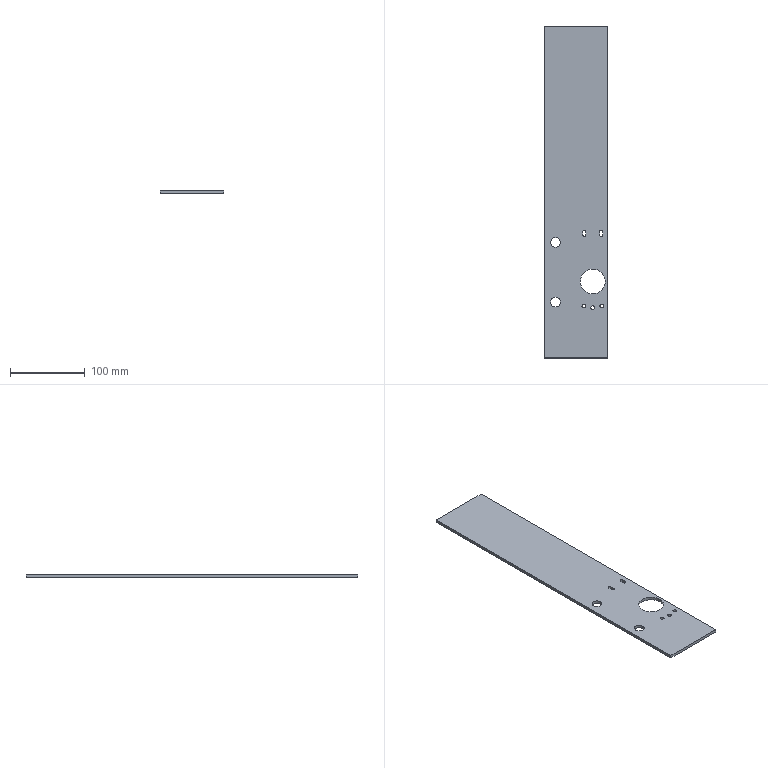Part | SolidWorks | features Extrusion 1 | 1 solid | 26 faces | box 85 x 445 x 4 mm | volume 146216 mm3 | cylinder 16 | plane 10 | commonest cylinder face diameters 5 x6 4 x4 13 x4 33.5 x2
STEP:
#1=CARTESIAN_POINT('',(48.25,-342.5,4.));
#2=VERTEX_POINT('',#1);
#3=CARTESIAN_POINT('',(81.75,-342.5,4.));
#4=VERTEX_POINT('',#3);
#5=CARTESIAN_POINT('',(65.,-342.5,4.));
#6=DIRECTION('',(0.,0.,1.));
#7=DIRECTION('',(1.,0.,0.));
#8=AXIS2_PLACEMENT_3D('',#5,#6,#7);
#9=CIRCLE('',#8,16.75);
#10=EDGE_CURVE('',#2,#4,#9,.T.);
#11=ORIENTED_EDGE('',*,*,#10,.T.);
#12=CARTESIAN_POINT('',(81.75,-342.5,0.));
#13=VERTEX_POINT('',#12);
#14=CARTESIAN_POINT('',(81.75,-342.5,4.));
#15=DIRECTION('',(0.,0.,-1.));
#16=VECTOR('',#15,1000.);
#17=LINE('',#14,#16);
#18=EDGE_CURVE('',#4,#13,#17,.T.);
#19=ORIENTED_EDGE('',*,*,#18,.T.);
#20=CARTESIAN_POINT('',(48.25,-342.5,0.));
#21=VERTEX_POINT('',#20);
#22=CARTESIAN_POINT('',(65.,-342.5,0.));
#23=DIRECTION('',(0.,0.,1.));
#24=DIRECTION('',(1.,0.,0.));
#25=AXIS2_PLACEMENT_3D('',#22,#23,#24);
#26=CIRCLE('',#25,16.75);
#27=EDGE_CURVE('',#21,#13,#26,.T.);
#28=ORIENTED_EDGE('',*,*,#27,.F.);
#29=CARTESIAN_POINT('',(48.25,-342.5,4.));
#30=DIRECTION('',(0.,0.,-1.));
#31=VECTOR('',#30,1000.);
#32=LINE('',#29,#31);
#33=EDGE_CURVE('',#2,#21,#32,.T.);
#34=ORIENTED_EDGE('',*,*,#33,.F.);
#35=EDGE_LOOP('',(#11,#19,#28,#34));
#36=FACE_OUTER_BOUND('',#35,.T.);
#37=CARTESIAN_POINT('',(65.,-342.5,4.));
#38=DIRECTION('',(0.,0.,-1.));
#39=DIRECTION('',(-1.,0.,0.));
#40=AXIS2_PLACEMENT_3D('',#37,#38,#39);
#41=CYLINDRICAL_SURFACE('',#40,16.75);
#42=ADVANCED_FACE('',(#36),#41,.F.);
#43=CARTESIAN_POINT('',(50.529,-375.389,4.));
#44=VERTEX_POINT('',#43);
#45=CARTESIAN_POINT('',(55.529,-375.389,4.));
#46=VERTEX_POINT('',#45);
#47=CARTESIAN_POINT('',(53.029,-375.389,4.));
#48=DIRECTION('',(0.,0.,1.));
#49=DIRECTION('',(1.,0.,0.));
#50=AXIS2_PLACEMENT_3D('',#47,#48,#49);
#51=CIRCLE('',#50,2.5);
#52=EDGE_CURVE('',#44,#46,#51,.T.);
#53=ORIENTED_EDGE('',*,*,#52,.T.);
#54=CARTESIAN_POINT('',(55.529,-375.389,0.));
#55=VERTEX_POINT('',#54);
#56=CARTESIAN_POINT('',(55.529,-375.389,4.));
#57=DIRECTION('',(0.,0.,-1.));
#58=VECTOR('',#57,1000.);
#59=LINE('',#56,#58);
#60=EDGE_CURVE('',#46,#55,#59,.T.);
#61=ORIENTED_EDGE('',*,*,#60,.T.);
#62=CARTESIAN_POINT('',(50.529,-375.389,0.));
#63=VERTEX_POINT('',#62);
#64=CARTESIAN_POINT('',(53.029,-375.389,0.));
#65=DIRECTION('',(0.,0.,1.));
#66=DIRECTION('',(1.,0.,0.));
#67=AXIS2_PLACEMENT_3D('',#64,#65,#66);
#68=CIRCLE('',#67,2.5);
#69=EDGE_CURVE('',#63,#55,#68,.T.);
#70=ORIENTED_EDGE('',*,*,#69,.F.);
#71=CARTESIAN_POINT('',(50.529,-375.389,4.));
#72=DIRECTION('',(0.,0.,-1.));
#73=VECTOR('',#72,1000.);
#74=LINE('',#71,#73);
#75=EDGE_CURVE('',#44,#63,#74,.T.);
#76=ORIENTED_EDGE('',*,*,#75,.F.);
#77=EDGE_LOOP('',(#53,#61,#70,#76));
#78=FACE_OUTER_BOUND('',#77,.T.);
#79=CARTESIAN_POINT('',(53.029,-375.389,4.));
#80=DIRECTION('',(0.,0.,-1.));
#81=DIRECTION('',(-1.,0.,0.));
#82=AXIS2_PLACEMENT_3D('',#79,#80,#81);
#83=CYLINDRICAL_SURFACE('',#82,2.5);
#84=ADVANCED_FACE('',(#78),#83,.F.);
#85=CARTESIAN_POINT('',(8.5,-290.,4.));
#86=VERTEX_POINT('',#85);
#87=CARTESIAN_POINT('',(21.5,-290.,4.));
#88=VERTEX_POINT('',#87);
#89=CARTESIAN_POINT('',(15.,-290.,4.));
#90=DIRECTION('',(0.,0.,1.));
#91=DIRECTION('',(1.,0.,0.));
#92=AXIS2_PLACEMENT_3D('',#89,#90,#91);
#93=CIRCLE('',#92,6.5);
#94=EDGE_CURVE('',#86,#88,#93,.T.);
#95=ORIENTED_EDGE('',*,*,#94,.T.);
#96=CARTESIAN_POINT('',(21.5,-290.,0.));
#97=VERTEX_POINT('',#96);
#98=CARTESIAN_POINT('',(21.5,-290.,4.));
#99=DIRECTION('',(0.,0.,-1.));
#100=VECTOR('',#99,1000.);
#101=LINE('',#98,#100);
#102=EDGE_CURVE('',#88,#97,#101,.T.);
#103=ORIENTED_EDGE('',*,*,#102,.T.);
#104=CARTESIAN_POINT('',(8.5,-290.,0.));
#105=VERTEX_POINT('',#104);
#106=CARTESIAN_POINT('',(15.,-290.,0.));
#107=DIRECTION('',(0.,0.,1.));
#108=DIRECTION('',(1.,0.,0.));
#109=AXIS2_PLACEMENT_3D('',#106,#107,#108);
#110=CIRCLE('',#109,6.5);
#111=EDGE_CURVE('',#105,#97,#110,.T.);
#112=ORIENTED_EDGE('',*,*,#111,.F.);
#113=CARTESIAN_POINT('',(8.5,-290.,4.));
#114=DIRECTION('',(0.,0.,-1.));
#115=VECTOR('',#114,1000.);
#116=LINE('',#113,#115);
#117=EDGE_CURVE('',#86,#105,#116,.T.);
#118=ORIENTED_EDGE('',*,*,#117,.F.);
#119=EDGE_LOOP('',(#95,#103,#112,#118));
#120=FACE_OUTER_BOUND('',#119,.T.);
#121=CARTESIAN_POINT('',(15.,-290.,4.));
#122=DIRECTION('',(0.,0.,-1.));
#123=DIRECTION('',(-1.,0.,0.));
#124=AXIS2_PLACEMENT_3D('',#121,#122,#123);
#125=CYLINDRICAL_SURFACE('',#124,6.5);
#126=ADVANCED_FACE('',(#120),#125,.F.);
#127=CARTESIAN_POINT('',(62.5,-377.5,4.));
#128=VERTEX_POINT('',#127);
#129=CARTESIAN_POINT('',(67.5,-377.5,4.));
#130=VERTEX_POINT('',#129);
#131=CARTESIAN_POINT('',(65.,-377.5,4.));
#132=DIRECTION('',(0.,0.,1.));
#133=DIRECTION('',(1.,0.,0.));
#134=AXIS2_PLACEMENT_3D('',#131,#132,#133);
#135=CIRCLE('',#134,2.5);
#136=EDGE_CURVE('',#128,#130,#135,.T.);
#137=ORIENTED_EDGE('',*,*,#136,.T.);
#138=CARTESIAN_POINT('',(67.5,-377.5,0.));
#139=VERTEX_POINT('',#138);
#140=CARTESIAN_POINT('',(67.5,-377.5,4.));
#141=DIRECTION('',(0.,0.,-1.));
#142=VECTOR('',#141,1000.);
#143=LINE('',#140,#142);
#144=EDGE_CURVE('',#130,#139,#143,.T.);
#145=ORIENTED_EDGE('',*,*,#144,.T.);
#146=CARTESIAN_POINT('',(62.5,-377.5,0.));
#147=VERTEX_POINT('',#146);
#148=CARTESIAN_POINT('',(65.,-377.5,0.));
#149=DIRECTION('',(0.,0.,1.));
#150=DIRECTION('',(1.,0.,0.));
#151=AXIS2_PLACEMENT_3D('',#148,#149,#150);
#152=CIRCLE('',#151,2.5);
#153=EDGE_CURVE('',#147,#139,#152,.T.);
#154=ORIENTED_EDGE('',*,*,#153,.F.);
#155=CARTESIAN_POINT('',(62.5,-377.5,4.));
#156=DIRECTION('',(0.,0.,-1.));
#157=VECTOR('',#156,1000.);
#158=LINE('',#155,#157);
#159=EDGE_CURVE('',#128,#147,#158,.T.);
#160=ORIENTED_EDGE('',*,*,#159,.F.);
#161=EDGE_LOOP('',(#137,#145,#154,#160));
#162=FACE_OUTER_BOUND('',#161,.T.);
#163=CARTESIAN_POINT('',(65.,-377.5,4.));
#164=DIRECTION('',(0.,0.,-1.));
#165=DIRECTION('',(-1.,0.,0.));
#166=AXIS2_PLACEMENT_3D('',#163,#164,#165);
#167=CYLINDRICAL_SURFACE('',#166,2.5);
#168=ADVANCED_FACE('',(#162),#167,.F.);
#169=CARTESIAN_POINT('',(74.471,-375.389,4.));
#170=VERTEX_POINT('',#169);
#171=CARTESIAN_POINT('',(79.471,-375.389,4.));
#172=VERTEX_POINT('',#171);
#173=CARTESIAN_POINT('',(76.971,-375.389,4.));
#174=DIRECTION('',(0.,0.,1.));
#175=DIRECTION('',(1.,0.,0.));
#176=AXIS2_PLACEMENT_3D('',#173,#174,#175);
#177=CIRCLE('',#176,2.5);
#178=EDGE_CURVE('',#170,#172,#177,.T.);
#179=ORIENTED_EDGE('',*,*,#178,.T.);
#180=CARTESIAN_POINT('',(79.471,-375.389,0.));
#181=VERTEX_POINT('',#180);
#182=CARTESIAN_POINT('',(79.471,-375.389,4.));
#183=DIRECTION('',(0.,0.,-1.));
#184=VECTOR('',#183,1000.);
#185=LINE('',#182,#184);
#186=EDGE_CURVE('',#172,#181,#185,.T.);
#187=ORIENTED_EDGE('',*,*,#186,.T.);
#188=CARTESIAN_POINT('',(74.471,-375.389,0.));
#189=VERTEX_POINT('',#188);
#190=CARTESIAN_POINT('',(76.971,-375.389,0.));
#191=DIRECTION('',(0.,0.,1.));
#192=DIRECTION('',(1.,0.,0.));
#193=AXIS2_PLACEMENT_3D('',#190,#191,#192);
#194=CIRCLE('',#193,2.5);
#195=EDGE_CURVE('',#189,#181,#194,.T.);
#196=ORIENTED_EDGE('',*,*,#195,.F.);
#197=CARTESIAN_POINT('',(74.471,-375.389,4.));
#198=DIRECTION('',(0.,0.,-1.));
#199=VECTOR('',#198,1000.);
#200=LINE('',#197,#199);
#201=EDGE_CURVE('',#170,#189,#200,.T.);
#202=ORIENTED_EDGE('',*,*,#201,.F.);
#203=EDGE_LOOP('',(#179,#187,#196,#202));
#204=FACE_OUTER_BOUND('',#203,.T.);
#205=CARTESIAN_POINT('',(76.971,-375.389,4.));
#206=DIRECTION('',(0.,0.,-1.));
#207=DIRECTION('',(-1.,0.,0.));
#208=AXIS2_PLACEMENT_3D('',#205,#206,#207);
#209=CYLINDRICAL_SURFACE('',#208,2.5);
#210=ADVANCED_FACE('',(#204),#209,.F.);
#211=CARTESIAN_POINT('',(8.5,-370.,4.));
#212=VERTEX_POINT('',#211);
#213=CARTESIAN_POINT('',(21.5,-370.,4.));
#214=VERTEX_POINT('',#213);
#215=CARTESIAN_POINT('',(15.,-370.,4.));
#216=DIRECTION('',(0.,0.,1.));
#217=DIRECTION('',(1.,0.,0.));
#218=AXIS2_PLACEMENT_3D('',#215,#216,#217);
#219=CIRCLE('',#218,6.5);
#220=EDGE_CURVE('',#212,#214,#219,.T.);
#221=ORIENTED_EDGE('',*,*,#220,.T.);
#222=CARTESIAN_POINT('',(21.5,-370.,0.));
#223=VERTEX_POINT('',#222);
#224=CARTESIAN_POINT('',(21.5,-370.,4.));
#225=DIRECTION('',(0.,0.,-1.));
#226=VECTOR('',#225,1000.);
#227=LINE('',#224,#226);
#228=EDGE_CURVE('',#214,#223,#227,.T.);
#229=ORIENTED_EDGE('',*,*,#228,.T.);
#230=CARTESIAN_POINT('',(8.5,-370.,0.));
#231=VERTEX_POINT('',#230);
#232=CARTESIAN_POINT('',(15.,-370.,0.));
#233=DIRECTION('',(0.,0.,1.));
#234=DIRECTION('',(1.,0.,0.));
#235=AXIS2_PLACEMENT_3D('',#232,#233,#234);
#236=CIRCLE('',#235,6.5);
#237=EDGE_CURVE('',#231,#223,#236,.T.);
#238=ORIENTED_EDGE('',*,*,#237,.F.);
#239=CARTESIAN_POINT('',(8.5,-370.,4.));
#240=DIRECTION('',(0.,0.,-1.));
#241=VECTOR('',#240,1000.);
#242=LINE('',#239,#241);
#243=EDGE_CURVE('',#212,#231,#242,.T.);
#244=ORIENTED_EDGE('',*,*,#243,.F.);
#245=EDGE_LOOP('',(#221,#229,#238,#244));
#246=FACE_OUTER_BOUND('',#245,.T.);
#247=CARTESIAN_POINT('',(15.,-370.,4.));
#248=DIRECTION('',(0.,0.,-1.));
#249=DIRECTION('',(-1.,0.,0.));
#250=AXIS2_PLACEMENT_3D('',#247,#248,#249);
#251=CYLINDRICAL_SURFACE('',#250,6.5);
#252=ADVANCED_FACE('',(#246),#251,.F.);
#253=ORIENTED_EDGE('',*,*,#136,.F.);
#254=CARTESIAN_POINT('',(65.,-377.5,4.));
#255=DIRECTION('',(0.,0.,1.));
#256=DIRECTION('',(1.,0.,0.));
#257=AXIS2_PLACEMENT_3D('',#254,#255,#256);
#258=CIRCLE('',#257,2.5);
#259=EDGE_CURVE('',#130,#128,#258,.T.);
#260=ORIENTED_EDGE('',*,*,#259,.F.);
#261=EDGE_LOOP('',(#253,#260));
#262=FACE_BOUND('',#261,.T.);
#263=ORIENTED_EDGE('',*,*,#178,.F.);
#264=CARTESIAN_POINT('',(76.971,-375.389,4.));
#265=DIRECTION('',(0.,0.,1.));
#266=DIRECTION('',(1.,0.,0.));
#267=AXIS2_PLACEMENT_3D('',#264,#265,#266);
#268=CIRCLE('',#267,2.5);
#269=EDGE_CURVE('',#172,#170,#268,.T.);
#270=ORIENTED_EDGE('',*,*,#269,.F.);
#271=EDGE_LOOP('',(#263,#270));
#272=FACE_BOUND('',#271,.T.);
#273=ORIENTED_EDGE('',*,*,#220,.F.);
#274=CARTESIAN_POINT('',(15.,-370.,4.));
#275=DIRECTION('',(0.,0.,1.));
#276=DIRECTION('',(1.,0.,0.));
#277=AXIS2_PLACEMENT_3D('',#274,#275,#276);
#278=CIRCLE('',#277,6.5);
#279=EDGE_CURVE('',#214,#212,#278,.T.);
#280=ORIENTED_EDGE('',*,*,#279,.F.);
#281=EDGE_LOOP('',(#273,#280));
#282=FACE_BOUND('',#281,.T.);
#283=CARTESIAN_POINT('',(55.8,-275.5,4.));
#284=VERTEX_POINT('',#283);
#285=CARTESIAN_POINT('',(51.8,-275.5,4.));
#286=VERTEX_POINT('',#285);
#287=CARTESIAN_POINT('',(53.8,-275.5,4.));
#288=DIRECTION('',(0.,0.,1.));
#289=DIRECTION('',(1.,0.,0.));
#290=AXIS2_PLACEMENT_3D('',#287,#288,#289);
#291=CIRCLE('',#290,2.);
#292=EDGE_CURVE('',#284,#286,#291,.T.);
#293=ORIENTED_EDGE('',*,*,#292,.F.);
#294=CARTESIAN_POINT('',(55.8,-280.5,4.));
#295=VERTEX_POINT('',#294);
#296=CARTESIAN_POINT('',(55.8,-275.5,4.));
#297=DIRECTION('',(0.,1.,0.));
#298=VECTOR('',#297,1000.);
#299=LINE('',#296,#298);
#300=EDGE_CURVE('',#295,#284,#299,.T.);
#301=ORIENTED_EDGE('',*,*,#300,.F.);
#302=CARTESIAN_POINT('',(51.8,-280.5,4.));
#303=VERTEX_POINT('',#302);
#304=CARTESIAN_POINT('',(53.8,-280.5,4.));
#305=DIRECTION('',(0.,0.,1.));
#306=DIRECTION('',(1.,0.,0.));
#307=AXIS2_PLACEMENT_3D('',#304,#305,#306);
#308=CIRCLE('',#307,2.);
#309=EDGE_CURVE('',#303,#295,#308,.T.);
#310=ORIENTED_EDGE('',*,*,#309,.F.);
#311=CARTESIAN_POINT('',(51.8,-275.5,4.));
#312=DIRECTION('',(0.,-1.,0.));
#313=VECTOR('',#312,1000.);
#314=LINE('',#311,#313);
#315=EDGE_CURVE('',#286,#303,#314,.T.);
#316=ORIENTED_EDGE('',*,*,#315,.F.);
#317=EDGE_LOOP('',(#293,#301,#310,#316));
#318=FACE_BOUND('',#317,.T.);
#319=CARTESIAN_POINT('',(0.,0.,4.));
#320=VERTEX_POINT('',#319);
#321=CARTESIAN_POINT('',(0.,-445.,4.));
#322=VERTEX_POINT('',#321);
#323=CARTESIAN_POINT('',(0.,-445.,4.));
#324=DIRECTION('',(0.,-1.,0.));
#325=VECTOR('',#324,1000.);
#326=LINE('',#323,#325);
#327=EDGE_CURVE('',#320,#322,#326,.T.);
#328=ORIENTED_EDGE('',*,*,#327,.T.);
#329=CARTESIAN_POINT('',(85.,-445.,4.));
#330=VERTEX_POINT('',#329);
#331=CARTESIAN_POINT('',(85.,-445.,4.));
#332=DIRECTION('',(1.,0.,0.));
#333=VECTOR('',#332,1000.);
#334=LINE('',#331,#333);
#335=EDGE_CURVE('',#322,#330,#334,.T.);
#336=ORIENTED_EDGE('',*,*,#335,.T.);
#337=CARTESIAN_POINT('',(85.,0.,4.));
#338=VERTEX_POINT('',#337);
#339=CARTESIAN_POINT('',(85.,0.,4.));
#340=DIRECTION('',(0.,1.,0.));
#341=VECTOR('',#340,1000.);
#342=LINE('',#339,#341);
#343=EDGE_CURVE('',#330,#338,#342,.T.);
#344=ORIENTED_EDGE('',*,*,#343,.T.);
#345=CARTESIAN_POINT('',(0.,0.,4.));
#346=DIRECTION('',(-1.,0.,0.));
#347=VECTOR('',#346,1000.);
#348=LINE('',#345,#347);
#349=EDGE_CURVE('',#338,#320,#348,.T.);
#350=ORIENTED_EDGE('',*,*,#349,.T.);
#351=EDGE_LOOP('',(#328,#336,#344,#350));
#352=FACE_OUTER_BOUND('',#351,.T.);
#353=CARTESIAN_POINT('',(78.3,-275.5,4.));
#354=VERTEX_POINT('',#353);
#355=CARTESIAN_POINT('',(74.3,-275.5,4.));
#356=VERTEX_POINT('',#355);
#357=CARTESIAN_POINT('',(76.3,-275.5,4.));
#358=DIRECTION('',(0.,0.,1.));
#359=DIRECTION('',(1.,0.,0.));
#360=AXIS2_PLACEMENT_3D('',#357,#358,#359);
#361=CIRCLE('',#360,2.);
#362=EDGE_CURVE('',#354,#356,#361,.T.);
#363=ORIENTED_EDGE('',*,*,#362,.F.);
#364=CARTESIAN_POINT('',(78.3,-280.5,4.));
#365=VERTEX_POINT('',#364);
#366=CARTESIAN_POINT('',(78.3,-275.5,4.));
#367=DIRECTION('',(0.,1.,0.));
#368=VECTOR('',#367,1000.);
#369=LINE('',#366,#368);
#370=EDGE_CURVE('',#365,#354,#369,.T.);
#371=ORIENTED_EDGE('',*,*,#370,.F.);
#372=CARTESIAN_POINT('',(74.3,-280.5,4.));
#373=VERTEX_POINT('',#372);
#374=CARTESIAN_POINT('',(76.3,-280.5,4.));
#375=DIRECTION('',(0.,0.,1.));
#376=DIRECTION('',(1.,0.,0.));
#377=AXIS2_PLACEMENT_3D('',#374,#375,#376);
#378=CIRCLE('',#377,2.);
#379=EDGE_CURVE('',#373,#365,#378,.T.);
#380=ORIENTED_EDGE('',*,*,#379,.F.);
#381=CARTESIAN_POINT('',(74.3,-275.5,4.));
#382=DIRECTION('',(0.,-1.,0.));
#383=VECTOR('',#382,1000.);
#384=LINE('',#381,#383);
#385=EDGE_CURVE('',#356,#373,#384,.T.);
#386=ORIENTED_EDGE('',*,*,#385,.F.);
#387=EDGE_LOOP('',(#363,#371,#380,#386));
#388=FACE_BOUND('',#387,.T.);
#389=ORIENTED_EDGE('',*,*,#94,.F.);
#390=CARTESIAN_POINT('',(15.,-290.,4.));
#391=DIRECTION('',(0.,0.,1.));
#392=DIRECTION('',(1.,0.,0.));
#393=AXIS2_PLACEMENT_3D('',#390,#391,#392);
#394=CIRCLE('',#393,6.5);
#395=EDGE_CURVE('',#88,#86,#394,.T.);
#396=ORIENTED_EDGE('',*,*,#395,.F.);
#397=EDGE_LOOP('',(#389,#396));
#398=FACE_BOUND('',#397,.T.);
#399=ORIENTED_EDGE('',*,*,#52,.F.);
#400=CARTESIAN_POINT('',(53.029,-375.389,4.));
#401=DIRECTION('',(0.,0.,1.));
#402=DIRECTION('',(1.,0.,0.));
#403=AXIS2_PLACEMENT_3D('',#400,#401,#402);
#404=CIRCLE('',#403,2.5);
#405=EDGE_CURVE('',#46,#44,#404,.T.);
#406=ORIENTED_EDGE('',*,*,#405,.F.);
#407=EDGE_LOOP('',(#399,#406));
#408=FACE_BOUND('',#407,.T.);
#409=ORIENTED_EDGE('',*,*,#10,.F.);
#410=CARTESIAN_POINT('',(65.,-342.5,4.));
#411=DIRECTION('',(0.,0.,1.));
#412=DIRECTION('',(1.,0.,0.));
#413=AXIS2_PLACEMENT_3D('',#410,#411,#412);
#414=CIRCLE('',#413,16.75);
#415=EDGE_CURVE('',#4,#2,#414,.T.);
#416=ORIENTED_EDGE('',*,*,#415,.F.);
#417=EDGE_LOOP('',(#409,#416));
#418=FACE_BOUND('',#417,.T.);
#419=CARTESIAN_POINT('',(0.,0.,4.));
#420=DIRECTION('',(0.,0.,-1.));
#421=DIRECTION('',(-1.,0.,0.));
#422=AXIS2_PLACEMENT_3D('',#419,#420,#421);
#423=PLANE('',#422);
#424=ADVANCED_FACE('',(#262,#272,#282,#318,#352,#388,#398,#408,#418),#423,.F.);
#425=ORIENTED_EDGE('',*,*,#69,.T.);
#426=CARTESIAN_POINT('',(53.029,-375.389,0.));
#427=DIRECTION('',(0.,0.,1.));
#428=DIRECTION('',(1.,0.,0.));
#429=AXIS2_PLACEMENT_3D('',#426,#427,#428);
#430=CIRCLE('',#429,2.5);
#431=EDGE_CURVE('',#55,#63,#430,.T.);
#432=ORIENTED_EDGE('',*,*,#431,.T.);
#433=EDGE_LOOP('',(#425,#432));
#434=FACE_BOUND('',#433,.T.);
#435=CARTESIAN_POINT('',(78.3,-280.5,0.));
#436=VERTEX_POINT('',#435);
#437=CARTESIAN_POINT('',(78.3,-275.5,0.));
#438=VERTEX_POINT('',#437);
#439=CARTESIAN_POINT('',(78.3,-275.5,0.));
#440=DIRECTION('',(0.,1.,0.));
#441=VECTOR('',#440,1000.);
#442=LINE('',#439,#441);
#443=EDGE_CURVE('',#436,#438,#442,.T.);
#444=ORIENTED_EDGE('',*,*,#443,.T.);
#445=CARTESIAN_POINT('',(74.3,-275.5,0.));
#446=VERTEX_POINT('',#445);
#447=CARTESIAN_POINT('',(76.3,-275.5,0.));
#448=DIRECTION('',(0.,0.,1.));
#449=DIRECTION('',(1.,0.,0.));
#450=AXIS2_PLACEMENT_3D('',#447,#448,#449);
#451=CIRCLE('',#450,2.);
#452=EDGE_CURVE('',#438,#446,#451,.T.);
#453=ORIENTED_EDGE('',*,*,#452,.T.);
#454=CARTESIAN_POINT('',(74.3,-280.5,0.));
#455=VERTEX_POINT('',#454);
#456=CARTESIAN_POINT('',(74.3,-275.5,0.));
#457=DIRECTION('',(0.,-1.,0.));
#458=VECTOR('',#457,1000.);
#459=LINE('',#456,#458);
#460=EDGE_CURVE('',#446,#455,#459,.T.);
#461=ORIENTED_EDGE('',*,*,#460,.T.);
#462=CARTESIAN_POINT('',(76.3,-280.5,0.));
#463=DIRECTION('',(0.,0.,1.));
#464=DIRECTION('',(1.,0.,0.));
#465=AXIS2_PLACEMENT_3D('',#462,#463,#464);
#466=CIRCLE('',#465,2.);
#467=EDGE_CURVE('',#455,#436,#466,.T.);
#468=ORIENTED_EDGE('',*,*,#467,.T.);
#469=EDGE_LOOP('',(#444,#453,#461,#468));
#470=FACE_BOUND('',#469,.T.);
#471=ORIENTED_EDGE('',*,*,#153,.T.);
#472=CARTESIAN_POINT('',(65.,-377.5,0.));
#473=DIRECTION('',(0.,0.,1.));
#474=DIRECTION('',(1.,0.,0.));
#475=AXIS2_PLACEMENT_3D('',#472,#473,#474);
#476=CIRCLE('',#475,2.5);
#477=EDGE_CURVE('',#139,#147,#476,.T.);
#478=ORIENTED_EDGE('',*,*,#477,.T.);
#479=EDGE_LOOP('',(#471,#478));
#480=FACE_BOUND('',#479,.T.);
#481=ORIENTED_EDGE('',*,*,#237,.T.);
#482=CARTESIAN_POINT('',(15.,-370.,0.));
#483=DIRECTION('',(0.,0.,1.));
#484=DIRECTION('',(1.,0.,0.));
#485=AXIS2_PLACEMENT_3D('',#482,#483,#484);
#486=CIRCLE('',#485,6.5);
#487=EDGE_CURVE('',#223,#231,#486,.T.);
#488=ORIENTED_EDGE('',*,*,#487,.T.);
#489=EDGE_LOOP('',(#481,#488));
#490=FACE_BOUND('',#489,.T.);
#491=CARTESIAN_POINT('',(0.,0.,0.));
#492=VERTEX_POINT('',#491);
#493=CARTESIAN_POINT('',(0.,-445.,0.));
#494=VERTEX_POINT('',#493);
#495=CARTESIAN_POINT('',(0.,-445.,0.));
#496=DIRECTION('',(0.,-1.,0.));
#497=VECTOR('',#496,1000.);
#498=LINE('',#495,#497);
#499=EDGE_CURVE('',#492,#494,#498,.T.);
#500=ORIENTED_EDGE('',*,*,#499,.F.);
#501=CARTESIAN_POINT('',(85.,0.,0.));
#502=VERTEX_POINT('',#501);
#503=CARTESIAN_POINT('',(0.,0.,0.));
#504=DIRECTION('',(-1.,0.,0.));
#505=VECTOR('',#504,1000.);
#506=LINE('',#503,#505);
#507=EDGE_CURVE('',#502,#492,#506,.T.);
#508=ORIENTED_EDGE('',*,*,#507,.F.);
#509=CARTESIAN_POINT('',(85.,-445.,0.));
#510=VERTEX_POINT('',#509);
#511=CARTESIAN_POINT('',(85.,0.,0.));
#512=DIRECTION('',(0.,1.,0.));
#513=VECTOR('',#512,1000.);
#514=LINE('',#511,#513);
#515=EDGE_CURVE('',#510,#502,#514,.T.);
#516=ORIENTED_EDGE('',*,*,#515,.F.);
#517=CARTESIAN_POINT('',(85.,-445.,0.));
#518=DIRECTION('',(1.,0.,0.));
#519=VECTOR('',#518,1000.);
#520=LINE('',#517,#519);
#521=EDGE_CURVE('',#494,#510,#520,.T.);
#522=ORIENTED_EDGE('',*,*,#521,.F.);
#523=EDGE_LOOP('',(#500,#508,#516,#522));
#524=FACE_OUTER_BOUND('',#523,.T.);
#525=CARTESIAN_POINT('',(55.8,-280.5,0.));
#526=VERTEX_POINT('',#525);
#527=CARTESIAN_POINT('',(55.8,-275.5,0.));
#528=VERTEX_POINT('',#527);
#529=CARTESIAN_POINT('',(55.8,-275.5,0.));
#530=DIRECTION('',(0.,1.,0.));
#531=VECTOR('',#530,1000.);
#532=LINE('',#529,#531);
#533=EDGE_CURVE('',#526,#528,#532,.T.);
#534=ORIENTED_EDGE('',*,*,#533,.T.);
#535=CARTESIAN_POINT('',(51.8,-275.5,0.));
#536=VERTEX_POINT('',#535);
#537=CARTESIAN_POINT('',(53.8,-275.5,0.));
#538=DIRECTION('',(0.,0.,1.));
#539=DIRECTION('',(1.,0.,0.));
#540=AXIS2_PLACEMENT_3D('',#537,#538,#539);
#541=CIRCLE('',#540,2.);
#542=EDGE_CURVE('',#528,#536,#541,.T.);
#543=ORIENTED_EDGE('',*,*,#542,.T.);
#544=CARTESIAN_POINT('',(51.8,-280.5,0.));
#545=VERTEX_POINT('',#544);
#546=CARTESIAN_POINT('',(51.8,-275.5,0.));
#547=DIRECTION('',(0.,-1.,0.));
#548=VECTOR('',#547,1000.);
#549=LINE('',#546,#548);
#550=EDGE_CURVE('',#536,#545,#549,.T.);
#551=ORIENTED_EDGE('',*,*,#550,.T.);
#552=CARTESIAN_POINT('',(53.8,-280.5,0.));
#553=DIRECTION('',(0.,0.,1.));
#554=DIRECTION('',(1.,0.,0.));
#555=AXIS2_PLACEMENT_3D('',#552,#553,#554);
#556=CIRCLE('',#555,2.);
#557=EDGE_CURVE('',#545,#526,#556,.T.);
#558=ORIENTED_EDGE('',*,*,#557,.T.);
#559=EDGE_LOOP('',(#534,#543,#551,#558));
#560=FACE_BOUND('',#559,.T.);
#561=ORIENTED_EDGE('',*,*,#195,.T.);
#562=CARTESIAN_POINT('',(76.971,-375.389,0.));
#563=DIRECTION('',(0.,0.,1.));
#564=DIRECTION('',(1.,0.,0.));
#565=AXIS2_PLACEMENT_3D('',#562,#563,#564);
#566=CIRCLE('',#565,2.5);
#567=EDGE_CURVE('',#181,#189,#566,.T.);
#568=ORIENTED_EDGE('',*,*,#567,.T.);
#569=EDGE_LOOP('',(#561,#568));
#570=FACE_BOUND('',#569,.T.);
#571=ORIENTED_EDGE('',*,*,#111,.T.);
#572=CARTESIAN_POINT('',(15.,-290.,0.));
#573=DIRECTION('',(0.,0.,1.));
#574=DIRECTION('',(1.,0.,0.));
#575=AXIS2_PLACEMENT_3D('',#572,#573,#574);
#576=CIRCLE('',#575,6.5);
#577=EDGE_CURVE('',#97,#105,#576,.T.);
#578=ORIENTED_EDGE('',*,*,#577,.T.);
#579=EDGE_LOOP('',(#571,#578));
#580=FACE_BOUND('',#579,.T.);
#581=ORIENTED_EDGE('',*,*,#27,.T.);
#582=CARTESIAN_POINT('',(65.,-342.5,0.));
#583=DIRECTION('',(0.,0.,1.));
#584=DIRECTION('',(1.,0.,0.));
#585=AXIS2_PLACEMENT_3D('',#582,#583,#584);
#586=CIRCLE('',#585,16.75);
#587=EDGE_CURVE('',#13,#21,#586,.T.);
#588=ORIENTED_EDGE('',*,*,#587,.T.);
#589=EDGE_LOOP('',(#581,#588));
#590=FACE_BOUND('',#589,.T.);
#591=CARTESIAN_POINT('',(0.,0.,0.));
#592=DIRECTION('',(0.,0.,-1.));
#593=DIRECTION('',(-1.,0.,0.));
#594=AXIS2_PLACEMENT_3D('',#591,#592,#593);
#595=PLANE('',#594);
#596=ADVANCED_FACE('',(#434,#470,#480,#490,#524,#560,#570,#580,#590),#595,.T.);
#597=ORIENTED_EDGE('',*,*,#499,.T.);
#598=CARTESIAN_POINT('',(0.,-445.,4.));
#599=DIRECTION('',(0.,0.,-1.));
#600=VECTOR('',#599,1000.);
#601=LINE('',#598,#600);
#602=EDGE_CURVE('',#322,#494,#601,.T.);
#603=ORIENTED_EDGE('',*,*,#602,.F.);
#604=ORIENTED_EDGE('',*,*,#327,.F.);
#605=CARTESIAN_POINT('',(0.,0.,4.));
#606=DIRECTION('',(0.,0.,-1.));
#607=VECTOR('',#606,1000.);
#608=LINE('',#605,#607);
#609=EDGE_CURVE('',#320,#492,#608,.T.);
#610=ORIENTED_EDGE('',*,*,#609,.T.);
#611=EDGE_LOOP('',(#597,#603,#604,#610));
#612=FACE_OUTER_BOUND('',#611,.T.);
#613=CARTESIAN_POINT('',(0.,-445.,4.));
#614=DIRECTION('',(1.,0.,0.));
#615=DIRECTION('',(0.,0.,-1.));
#616=AXIS2_PLACEMENT_3D('',#613,#614,#615);
#617=PLANE('',#616);
#618=ADVANCED_FACE('',(#612),#617,.F.);
#619=ORIENTED_EDGE('',*,*,#521,.T.);
#620=CARTESIAN_POINT('',(85.,-445.,4.));
#621=DIRECTION('',(0.,0.,-1.));
#622=VECTOR('',#621,1000.);
#623=LINE('',#620,#622);
#624=EDGE_CURVE('',#330,#510,#623,.T.);
#625=ORIENTED_EDGE('',*,*,#624,.F.);
#626=ORIENTED_EDGE('',*,*,#335,.F.);
#627=ORIENTED_EDGE('',*,*,#602,.T.);
#628=EDGE_LOOP('',(#619,#625,#626,#627));
#629=FACE_OUTER_BOUND('',#628,.T.);
#630=CARTESIAN_POINT('',(85.,-445.,4.));
#631=DIRECTION('',(0.,1.,0.));
#632=DIRECTION('',(0.,0.,1.));
#633=AXIS2_PLACEMENT_3D('',#630,#631,#632);
#634=PLANE('',#633);
#635=ADVANCED_FACE('',(#629),#634,.F.);
#636=ORIENTED_EDGE('',*,*,#515,.T.);
#637=CARTESIAN_POINT('',(85.,0.,4.));
#638=DIRECTION('',(0.,0.,-1.));
#639=VECTOR('',#638,1000.);
#640=LINE('',#637,#639);
#641=EDGE_CURVE('',#338,#502,#640,.T.);
#642=ORIENTED_EDGE('',*,*,#641,.F.);
#643=ORIENTED_EDGE('',*,*,#343,.F.);
#644=ORIENTED_EDGE('',*,*,#624,.T.);
#645=EDGE_LOOP('',(#636,#642,#643,#644));
#646=FACE_OUTER_BOUND('',#645,.T.);
#647=CARTESIAN_POINT('',(85.,0.,4.));
#648=DIRECTION('',(-1.,0.,0.));
#649=DIRECTION('',(0.,0.,1.));
#650=AXIS2_PLACEMENT_3D('',#647,#648,#649);
#651=PLANE('',#650);
#652=ADVANCED_FACE('',(#646),#651,.F.);
#653=ORIENTED_EDGE('',*,*,#507,.T.);
#654=ORIENTED_EDGE('',*,*,#609,.F.);
#655=ORIENTED_EDGE('',*,*,#349,.F.);
#656=ORIENTED_EDGE('',*,*,#641,.T.);
#657=EDGE_LOOP('',(#653,#654,#655,#656));
#658=FACE_OUTER_BOUND('',#657,.T.);
#659=CARTESIAN_POINT('',(0.,0.,4.));
#660=DIRECTION('',(0.,-1.,0.));
#661=DIRECTION('',(0.,0.,-1.));
#662=AXIS2_PLACEMENT_3D('',#659,#660,#661);
#663=PLANE('',#662);
#664=ADVANCED_FACE('',(#658),#663,.F.);
#665=ORIENTED_EDGE('',*,*,#542,.F.);
#666=CARTESIAN_POINT('',(55.8,-275.5,4.));
#667=DIRECTION('',(0.,0.,-1.));
#668=VECTOR('',#667,1000.);
#669=LINE('',#666,#668);
#670=EDGE_CURVE('',#284,#528,#669,.T.);
#671=ORIENTED_EDGE('',*,*,#670,.F.);
#672=ORIENTED_EDGE('',*,*,#292,.T.);
#673=CARTESIAN_POINT('',(51.8,-275.5,4.));
#674=DIRECTION('',(0.,0.,-1.));
#675=VECTOR('',#674,1000.);
#676=LINE('',#673,#675);
#677=EDGE_CURVE('',#286,#536,#676,.T.);
#678=ORIENTED_EDGE('',*,*,#677,.T.);
#679=EDGE_LOOP('',(#665,#671,#672,#678));
#680=FACE_OUTER_BOUND('',#679,.T.);
#681=CARTESIAN_POINT('',(53.8,-275.5,4.));
#682=DIRECTION('',(0.,0.,-1.));
#683=DIRECTION('',(-1.,0.,0.));
#684=AXIS2_PLACEMENT_3D('',#681,#682,#683);
#685=CYLINDRICAL_SURFACE('',#684,2.);
#686=ADVANCED_FACE('',(#680),#685,.F.);
#687=ORIENTED_EDGE('',*,*,#550,.F.);
#688=ORIENTED_EDGE('',*,*,#677,.F.);
#689=ORIENTED_EDGE('',*,*,#315,.T.);
#690=CARTESIAN_POINT('',(51.8,-280.5,4.));
#691=DIRECTION('',(0.,0.,-1.));
#692=VECTOR('',#691,1000.);
#693=LINE('',#690,#692);
#694=EDGE_CURVE('',#303,#545,#693,.T.);
#695=ORIENTED_EDGE('',*,*,#694,.T.);
#696=EDGE_LOOP('',(#687,#688,#689,#695));
#697=FACE_OUTER_BOUND('',#696,.T.);
#698=CARTESIAN_POINT('',(51.8,-275.5,4.));
#699=DIRECTION('',(1.,0.,0.));
#700=DIRECTION('',(0.,0.,-1.));
#701=AXIS2_PLACEMENT_3D('',#698,#699,#700);
#702=PLANE('',#701);
#703=ADVANCED_FACE('',(#697),#702,.T.);
#704=ORIENTED_EDGE('',*,*,#557,.F.);
#705=ORIENTED_EDGE('',*,*,#694,.F.);
#706=ORIENTED_EDGE('',*,*,#309,.T.);
#707=CARTESIAN_POINT('',(55.8,-280.5,4.));
#708=DIRECTION('',(0.,0.,-1.));
#709=VECTOR('',#708,1000.);
#710=LINE('',#707,#709);
#711=EDGE_CURVE('',#295,#526,#710,.T.);
#712=ORIENTED_EDGE('',*,*,#711,.T.);
#713=EDGE_LOOP('',(#704,#705,#706,#712));
#714=FACE_OUTER_BOUND('',#713,.T.);
#715=CARTESIAN_POINT('',(53.8,-280.5,4.));
#716=DIRECTION('',(0.,0.,-1.));
#717=DIRECTION('',(-1.,0.,0.));
#718=AXIS2_PLACEMENT_3D('',#715,#716,#717);
#719=CYLINDRICAL_SURFACE('',#718,2.);
#720=ADVANCED_FACE('',(#714),#719,.F.);
#721=ORIENTED_EDGE('',*,*,#533,.F.);
#722=ORIENTED_EDGE('',*,*,#711,.F.);
#723=ORIENTED_EDGE('',*,*,#300,.T.);
#724=ORIENTED_EDGE('',*,*,#670,.T.);
#725=EDGE_LOOP('',(#721,#722,#723,#724));
#726=FACE_OUTER_BOUND('',#725,.T.);
#727=CARTESIAN_POINT('',(55.8,-275.5,4.));
#728=DIRECTION('',(-1.,0.,0.));
#729=DIRECTION('',(0.,-1.,0.));
#730=AXIS2_PLACEMENT_3D('',#727,#728,#729);
#731=PLANE('',#730);
#732=ADVANCED_FACE('',(#726),#731,.T.);
#733=ORIENTED_EDGE('',*,*,#228,.F.);
#734=ORIENTED_EDGE('',*,*,#279,.T.);
#735=ORIENTED_EDGE('',*,*,#243,.T.);
#736=ORIENTED_EDGE('',*,*,#487,.F.);
#737=EDGE_LOOP('',(#733,#734,#735,#736));
#738=FACE_OUTER_BOUND('',#737,.T.);
#739=CARTESIAN_POINT('',(15.,-370.,4.));
#740=DIRECTION('',(0.,0.,-1.));
#741=DIRECTION('',(-1.,0.,0.));
#742=AXIS2_PLACEMENT_3D('',#739,#740,#741);
#743=CYLINDRICAL_SURFACE('',#742,6.5);
#744=ADVANCED_FACE('',(#738),#743,.F.);
#745=ORIENTED_EDGE('',*,*,#186,.F.);
#746=ORIENTED_EDGE('',*,*,#269,.T.);
#747=ORIENTED_EDGE('',*,*,#201,.T.);
#748=ORIENTED_EDGE('',*,*,#567,.F.);
#749=EDGE_LOOP('',(#745,#746,#747,#748));
#750=FACE_OUTER_BOUND('',#749,.T.);
#751=CARTESIAN_POINT('',(76.971,-375.389,4.));
#752=DIRECTION('',(0.,0.,-1.));
#753=DIRECTION('',(-1.,0.,0.));
#754=AXIS2_PLACEMENT_3D('',#751,#752,#753);
#755=CYLINDRICAL_SURFACE('',#754,2.5);
#756=ADVANCED_FACE('',(#750),#755,.F.);
#757=ORIENTED_EDGE('',*,*,#144,.F.);
#758=ORIENTED_EDGE('',*,*,#259,.T.);
#759=ORIENTED_EDGE('',*,*,#159,.T.);
#760=ORIENTED_EDGE('',*,*,#477,.F.);
#761=EDGE_LOOP('',(#757,#758,#759,#760));
#762=FACE_OUTER_BOUND('',#761,.T.);
#763=CARTESIAN_POINT('',(65.,-377.5,4.));
#764=DIRECTION('',(0.,0.,-1.));
#765=DIRECTION('',(-1.,0.,0.));
#766=AXIS2_PLACEMENT_3D('',#763,#764,#765);
#767=CYLINDRICAL_SURFACE('',#766,2.5);
#768=ADVANCED_FACE('',(#762),#767,.F.);
#769=ORIENTED_EDGE('',*,*,#452,.F.);
#770=CARTESIAN_POINT('',(78.3,-275.5,4.));
#771=DIRECTION('',(0.,0.,-1.));
#772=VECTOR('',#771,1000.);
#773=LINE('',#770,#772);
#774=EDGE_CURVE('',#354,#438,#773,.T.);
#775=ORIENTED_EDGE('',*,*,#774,.F.);
#776=ORIENTED_EDGE('',*,*,#362,.T.);
#777=CARTESIAN_POINT('',(74.3,-275.5,4.));
#778=DIRECTION('',(0.,0.,-1.));
#779=VECTOR('',#778,1000.);
#780=LINE('',#777,#779);
#781=EDGE_CURVE('',#356,#446,#780,.T.);
#782=ORIENTED_EDGE('',*,*,#781,.T.);
#783=EDGE_LOOP('',(#769,#775,#776,#782));
#784=FACE_OUTER_BOUND('',#783,.T.);
#785=CARTESIAN_POINT('',(76.3,-275.5,4.));
#786=DIRECTION('',(0.,0.,-1.));
#787=DIRECTION('',(-1.,0.,0.));
#788=AXIS2_PLACEMENT_3D('',#785,#786,#787);
#789=CYLINDRICAL_SURFACE('',#788,2.);
#790=ADVANCED_FACE('',(#784),#789,.F.);
#791=ORIENTED_EDGE('',*,*,#460,.F.);
#792=ORIENTED_EDGE('',*,*,#781,.F.);
#793=ORIENTED_EDGE('',*,*,#385,.T.);
#794=CARTESIAN_POINT('',(74.3,-280.5,4.));
#795=DIRECTION('',(0.,0.,-1.));
#796=VECTOR('',#795,1000.);
#797=LINE('',#794,#796);
#798=EDGE_CURVE('',#373,#455,#797,.T.);
#799=ORIENTED_EDGE('',*,*,#798,.T.);
#800=EDGE_LOOP('',(#791,#792,#793,#799));
#801=FACE_OUTER_BOUND('',#800,.T.);
#802=CARTESIAN_POINT('',(74.3,-275.5,4.));
#803=DIRECTION('',(1.,0.,0.));
#804=DIRECTION('',(0.,0.,-1.));
#805=AXIS2_PLACEMENT_3D('',#802,#803,#804);
#806=PLANE('',#805);
#807=ADVANCED_FACE('',(#801),#806,.T.);
#808=ORIENTED_EDGE('',*,*,#467,.F.);
#809=ORIENTED_EDGE('',*,*,#798,.F.);
#810=ORIENTED_EDGE('',*,*,#379,.T.);
#811=CARTESIAN_POINT('',(78.3,-280.5,4.));
#812=DIRECTION('',(0.,0.,-1.));
#813=VECTOR('',#812,1000.);
#814=LINE('',#811,#813);
#815=EDGE_CURVE('',#365,#436,#814,.T.);
#816=ORIENTED_EDGE('',*,*,#815,.T.);
#817=EDGE_LOOP('',(#808,#809,#810,#816));
#818=FACE_OUTER_BOUND('',#817,.T.);
#819=CARTESIAN_POINT('',(76.3,-280.5,4.));
#820=DIRECTION('',(0.,0.,-1.));
#821=DIRECTION('',(-1.,0.,0.));
#822=AXIS2_PLACEMENT_3D('',#819,#820,#821);
#823=CYLINDRICAL_SURFACE('',#822,2.);
#824=ADVANCED_FACE('',(#818),#823,.F.);
#825=ORIENTED_EDGE('',*,*,#443,.F.);
#826=ORIENTED_EDGE('',*,*,#815,.F.);
#827=ORIENTED_EDGE('',*,*,#370,.T.);
#828=ORIENTED_EDGE('',*,*,#774,.T.);
#829=EDGE_LOOP('',(#825,#826,#827,#828));
#830=FACE_OUTER_BOUND('',#829,.T.);
#831=CARTESIAN_POINT('',(78.3,-275.5,4.));
#832=DIRECTION('',(-1.,0.,0.));
#833=DIRECTION('',(0.,0.,1.));
#834=AXIS2_PLACEMENT_3D('',#831,#832,#833);
#835=PLANE('',#834);
#836=ADVANCED_FACE('',(#830),#835,.T.);
#837=ORIENTED_EDGE('',*,*,#102,.F.);
#838=ORIENTED_EDGE('',*,*,#395,.T.);
#839=ORIENTED_EDGE('',*,*,#117,.T.);
#840=ORIENTED_EDGE('',*,*,#577,.F.);
#841=EDGE_LOOP('',(#837,#838,#839,#840));
#842=FACE_OUTER_BOUND('',#841,.T.);
#843=CARTESIAN_POINT('',(15.,-290.,4.));
#844=DIRECTION('',(0.,0.,-1.));
#845=DIRECTION('',(-1.,0.,0.));
#846=AXIS2_PLACEMENT_3D('',#843,#844,#845);
#847=CYLINDRICAL_SURFACE('',#846,6.5);
#848=ADVANCED_FACE('',(#842),#847,.F.);
#849=ORIENTED_EDGE('',*,*,#60,.F.);
#850=ORIENTED_EDGE('',*,*,#405,.T.);
#851=ORIENTED_EDGE('',*,*,#75,.T.);
#852=ORIENTED_EDGE('',*,*,#431,.F.);
#853=EDGE_LOOP('',(#849,#850,#851,#852));
#854=FACE_OUTER_BOUND('',#853,.T.);
#855=CARTESIAN_POINT('',(53.029,-375.389,4.));
#856=DIRECTION('',(0.,0.,-1.));
#857=DIRECTION('',(-1.,0.,0.));
#858=AXIS2_PLACEMENT_3D('',#855,#856,#857);
#859=CYLINDRICAL_SURFACE('',#858,2.5);
#860=ADVANCED_FACE('',(#854),#859,.F.);
#861=ORIENTED_EDGE('',*,*,#18,.F.);
#862=ORIENTED_EDGE('',*,*,#415,.T.);
#863=ORIENTED_EDGE('',*,*,#33,.T.);
#864=ORIENTED_EDGE('',*,*,#587,.F.);
#865=EDGE_LOOP('',(#861,#862,#863,#864));
#866=FACE_OUTER_BOUND('',#865,.T.);
#867=CARTESIAN_POINT('',(65.,-342.5,4.));
#868=DIRECTION('',(0.,0.,-1.));
#869=DIRECTION('',(-1.,0.,0.));
#870=AXIS2_PLACEMENT_3D('',#867,#868,#869);
#871=CYLINDRICAL_SURFACE('',#870,16.75);
#872=ADVANCED_FACE('',(#866),#871,.F.);
#873=CLOSED_SHELL('',(#42,#84,#126,#168,#210,#252,#424,#596,#618,#635,#652,#664,#686,#703,#720,#732,#744,#756,#768,#790,#807,#824,#836,#848,#860,#872));
#874=MANIFOLD_SOLID_BREP('',#873);
#875=CARTESIAN_POINT('',(0.,0.,0.));
#876=DIRECTION('',(0.,0.,1.));
#877=DIRECTION('',(1.,0.,0.));
#878=AXIS2_PLACEMENT_3D('',#875,#876,#877);
#879=(LENGTH_UNIT()NAMED_UNIT(*)SI_UNIT(.MILLI.,.METRE.));
#880=UNCERTAINTY_MEASURE_WITH_UNIT(LENGTH_MEASURE(0.00001),#879,'','');
#881=(NAMED_UNIT(*)PLANE_ANGLE_UNIT()SI_UNIT($,.RADIAN.));
#882=(NAMED_UNIT(*)SI_UNIT($,.STERADIAN.)SOLID_ANGLE_UNIT());
#883=(GEOMETRIC_REPRESENTATION_CONTEXT(3)GLOBAL_UNCERTAINTY_ASSIGNED_CONTEXT((#880))GLOBAL_UNIT_ASSIGNED_CONTEXT((#879,#881,#882))REPRESENTATION_CONTEXT('',''));
#884=ADVANCED_BREP_SHAPE_REPRESENTATION('',(#874,#878),#883);